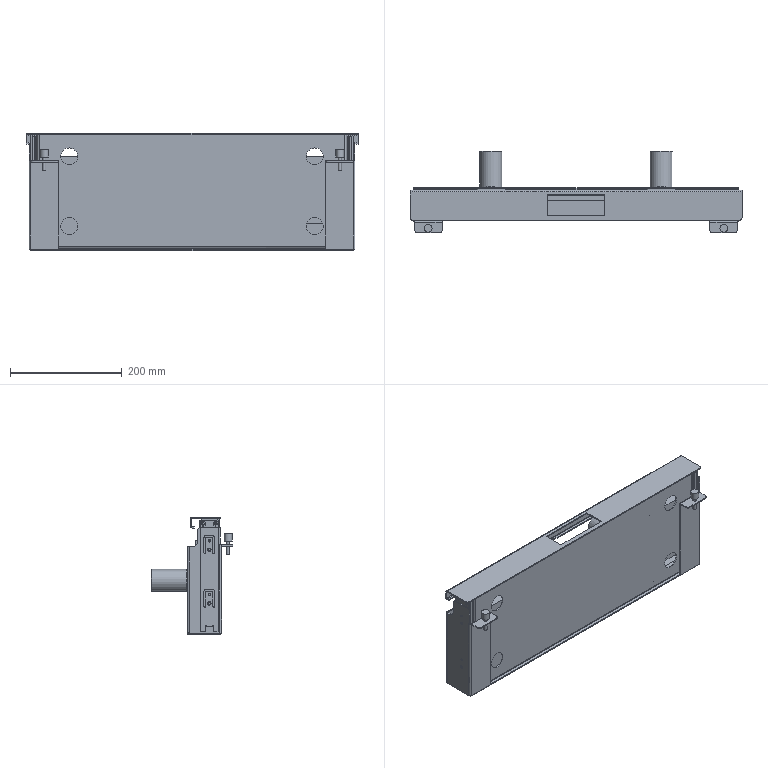Part | NX | 11 solids | 1034 faces | box 595 x 146 x 210 mm | volume 3219497 mm3 | plane 612 | cylinder 354 | spline 56 | cone 12 | commonest cylinder face diameters 2 x126 6 x54 4 x28 1 x24 5 x18 3 x14